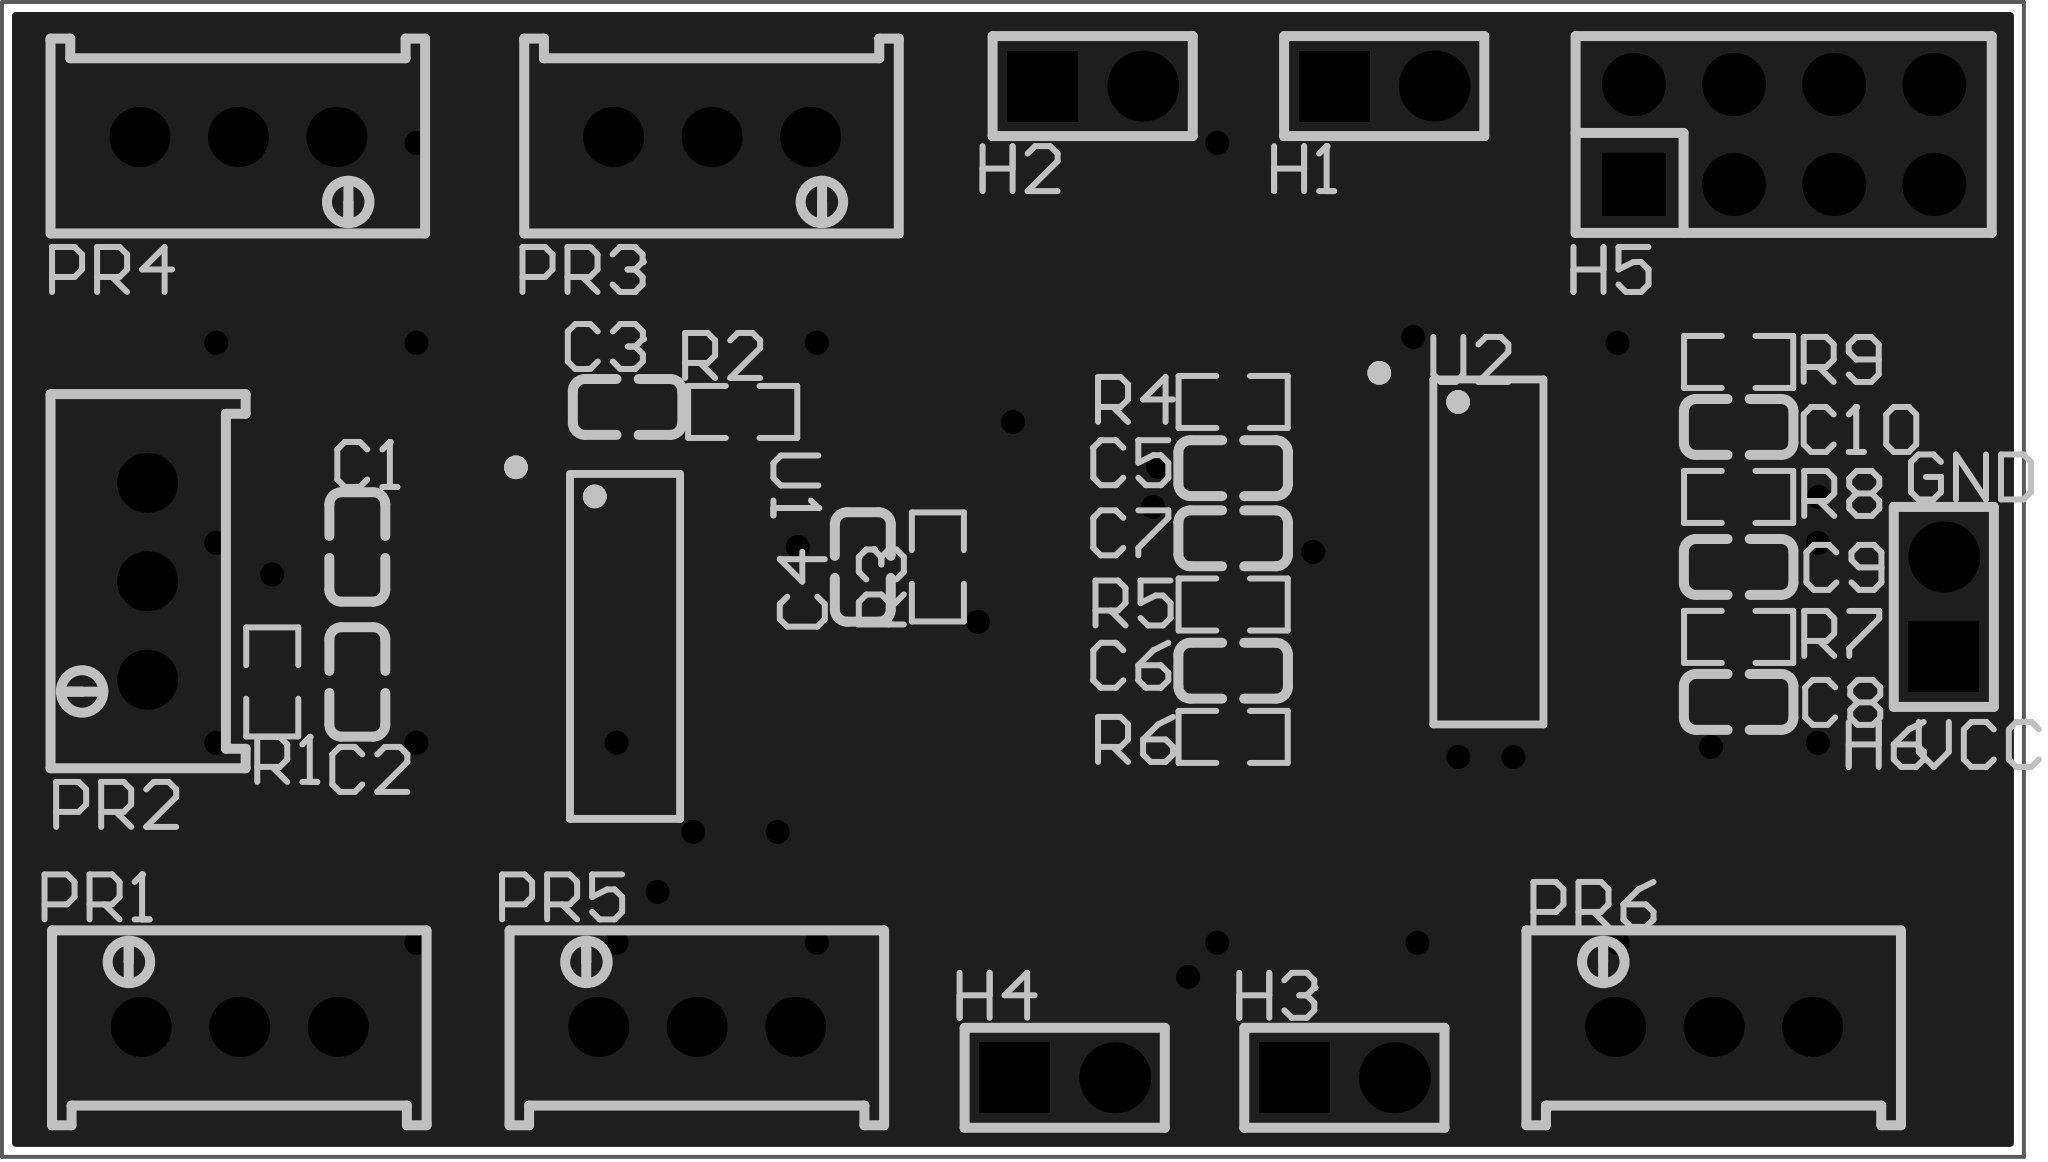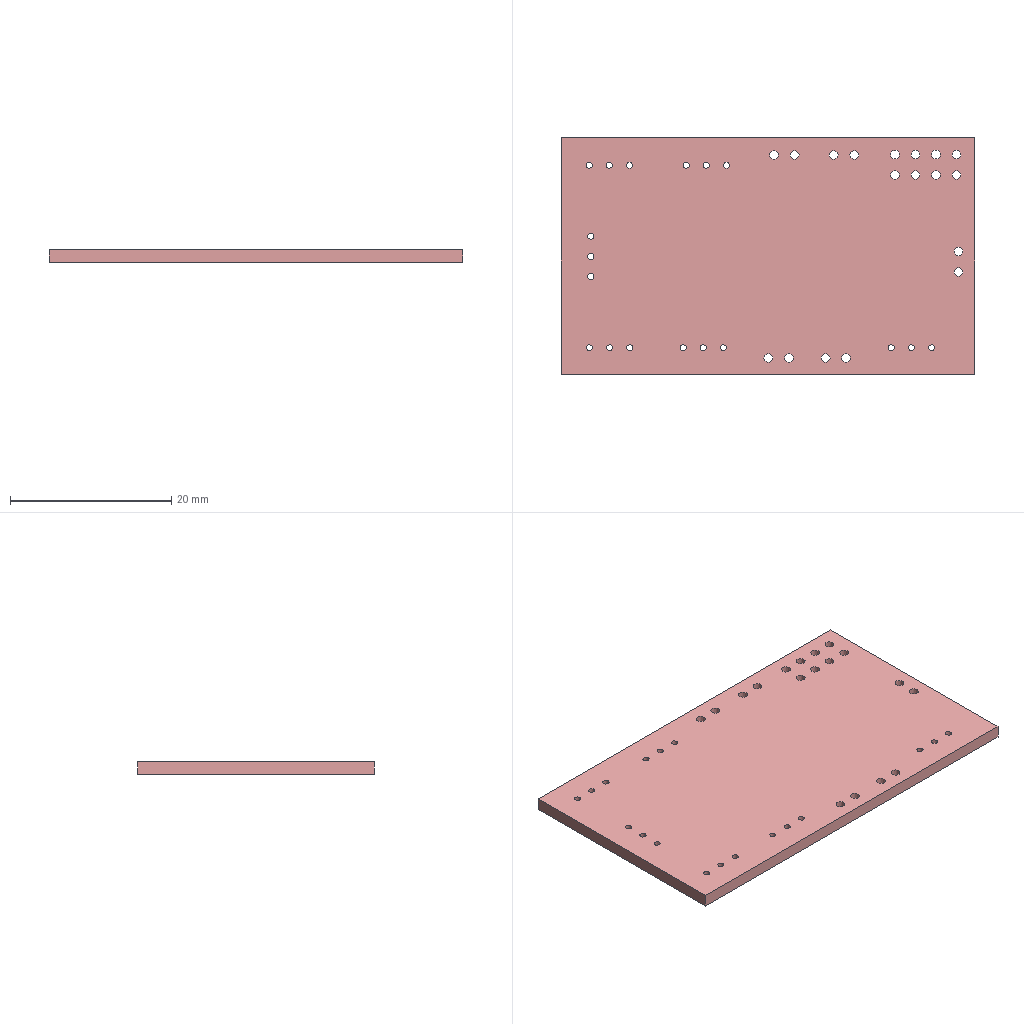Circuit board layout | Altium Designer | box 51.3 x 29.3 x 1.6 mm
Layer stack:
# Altium Designer layer stack of  (unit mm; dielectric type: 0 none, 1 core, 2 prepreg, 3 surface material)
index,name,kind,layer,copper_thickness_mm,dielectric_type,dielectric_thickness_mm,dielectric_material,dielectric_constant
0,Top Paste Mask Layer,other,,,,,,
1,Top Silkscreen Layer,other,,,,,,
2,Top Solder Mask Layer,dielectric,,,3,0.01,,3.3
3,Top Layer,copper,Top Layer,0.035,,,,
4,Dielectric1,dielectric,,,3,1.51,FR4,4.5
5,Bottom Layer,copper,Bottom Layer,0.035,,,,
6,Bottom Solder Mask Layer,dielectric,,,3,0.01,,3.3
7,Bottom Silkscreen Layer,other,,,,,,
8,Bottom Paste Mask Layer,other,,,,,,
# drill layer pairs: low layer,high layer
drill_pair,Top Layer,Bottom Layer
Part placement:
Designator,Comment,Layer,Footprint,Center-X(mm),Center-Y(mm),Rotation
C1,22nF,TopLayer,C0603,86.995,93.218,270
C2,22nF,TopLayer,C0603,86.995,89.789,270
C3,100PF,TopLayer,C0603,93.853,96.774,0
C4,1nF,TopLayer,C0603,99.822,92.71,90
C5,100nF,TopLayer,C0603,109.22,95.219,0
C6,100pF,TopLayer,C0603,109.22,90.074,0
C7,100pF,TopLayer,C0603,109.22,93.437,0
C8,100pF,TopLayer,C0603,122.047,89.281,180
C9,80pF,TopLayer,C0603,122.047,92.71,180
C10,500pF,TopLayer,C0603,122.047,96.266,0
H1,,TopLayer,HDR-TH_2P-P2.54-V-M-1,113.053,104.925,0
H2,,TopLayer,HDR-TH_2P-P2.54-V-M-1,105.655,104.925,0
H3,,TopLayer,HDR-TH_2P-P2.54-V-M-1,112.042,79.733,0
H4,,TopLayer,HDR-TH_2P-P2.54-V-M-1,104.945,79.733,0
H5,,TopLayer,HDR-TH_8P-P2.54-V-F-R2-C4-S2.54-1,123.19,103.695,0
H6,,TopLayer,HDR-TH_2P-P2.54-V-M-1,127.254,91.694,90
PR1,10kΩ,TopLayer,R_3296,83.998,81.026,0
PR2,10kΩ,TopLayer,R_3296,81.661,92.346,90
PR3,20kΩ,TopLayer,R_3296,95.985,103.632,180
PR4,10kΩ,TopLayer,R_3296,83.965,103.632,180
PR5,10kΩ,TopLayer,R_3296,95.608,81.026,0
PR6,100kΩ,TopLayer,R_3296,121.412,81.026,0
R1,1K,TopLayer,R0603,84.836,89.789,90
R2,10K,TopLayer,R0603,96.774,96.647,0
R3,1K,TopLayer,R0603,101.727,92.71,90
R4,100K,TopLayer,R0603,109.22,96.901,180
R5,100K,TopLayer,R0603,109.22,91.755,0
R6,200K,TopLayer,R0603,109.22,88.392,180
R7,100K,TopLayer,R0603,122.047,90.932,180
R8,40K,TopLayer,R0603,122.047,94.488,180
R9,100K,TopLayer,R0603,122.047,97.917,180
U1,SN74LS00DG4,TopLayer,SOIC-14_L8.7-W3.9-P1.27-LS6.0-BL,93.788,90.691,270
U2,LM324DT,TopLayer,SOIC-14_L8.7-W3.9-P1.27-LS6.0-BL,115.697,93.091,270
Pad and via stacks:
# Altium Designer via and pad stacks of  (unit mm). Each distinct definition once, with the count of objects using it.
# via: kind,start_layer,end_layer,hole_mm,diameter_mm,mode(0 simple;1 top-mid-bottom;2 full stack),diameter_per_layer,count,example_net
# pad: kind,layer,hole_mm,hole_type(0 round;1 square;2 slot),plating,top_size,top_shape(1 round;2 rect;3 octagon;9 rounded rect),mid_size,bottom_size,mode,footprint,size_per_layer,count,example
pad,Top Layer,0,0,plated,0.8x0.9,2,0.8x0.9,0.8x0.9,0,C0603,,20,C1.2
pad,Top Layer,0,0,plated,0.8065x0.864,2,0.8065x0.864,0.8065x0.864,0,R0603,,18,R1.2
pad,Top Layer,0,0,plated,0.574x2.038,1,0.574x2.038,0.574x2.038,0,SOIC-14_L8.7-W3.9-P1.27-LS6.0-BL,,28,U1.8
pad,Multi-Layer,1.1,0,plated,1.8x1.8,1,1.8x1.8,1.8x1.8,0,HDR-TH_2P-P2.54-V-M-1,,5,H1.2
pad,Multi-Layer,1.1,0,plated,1.8x1.8,2,1.8x1.8,1.8x1.8,0,HDR-TH_2P-P2.54-V-M-1,,5,H1.1
pad,Multi-Layer,1.1,0,plated,1.6x1.6,2,1.6x1.6,1.6x1.6,0,HDR-TH_8P-P2.54-V-F-R2-C4-S2.54-1,,1,H5.1
pad,Multi-Layer,1.1,0,plated,1.6x1.6,1,1.6x1.6,1.6x1.6,0,HDR-TH_8P-P2.54-V-F-R2-C4-S2.54-1,,7,H5.2
pad,Multi-Layer,0.762,0,plated,1.524x1.524,1,1.524x1.524,1.524x1.524,0,R_3296,,18,PR1.2
via,Top Layer,Bottom Layer,0.3048,0.61,0,,34,$1N12
Copper pours:
name,layer,net,type(0 solid;1 hatched;2 none)
Top Layer-GND,Top Layer,GND,0
Bottom Layer-GND,Bottom Layer,GND,0
Design rules, without the lines most boards share:
# Altium Designer design rules of  (exported by Altium Designer, unit mm)
# columns: name | kind | enabled | priority | scope1 | scope2 | descriptor | typed fields (field=value)
creepage | 65 | enabled | 1 | All | All | Creepage Distance Constraint =(0mil) (All),(All) |